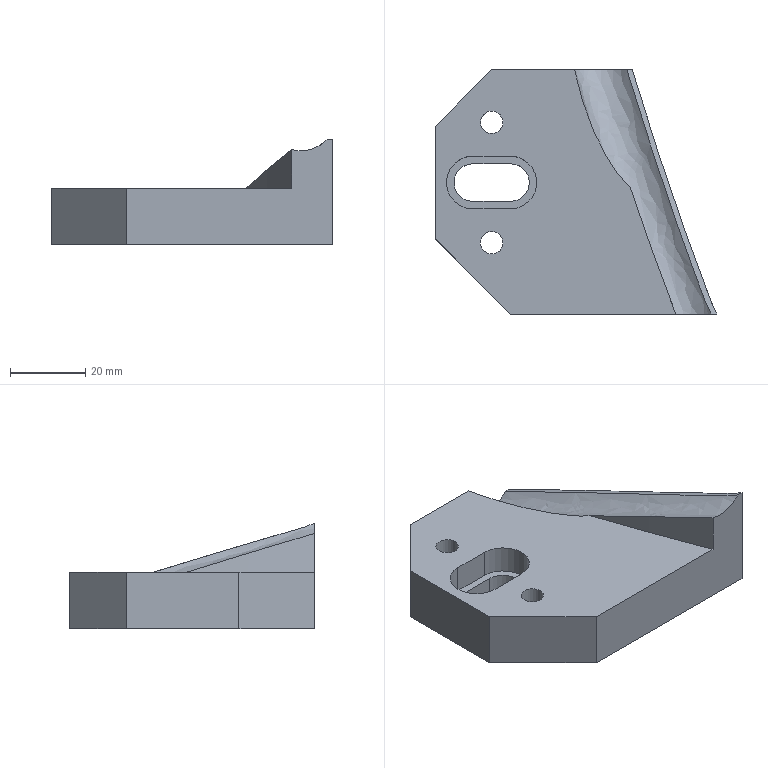Part | NX | features solid 2 | 1 solid | 22 faces | box 74.881 x 65 x 28.021 mm | volume 52689 mm3 | plane 12 | cylinder 6 | spline 4 | commonest cylinder face diameters 6 x2 10 x2 14 x2
STEP:
#1=CARTESIAN_POINT('',(-605.,-23.,-39.));
#2=VERTEX_POINT('',#1);
#3=CARTESIAN_POINT('',(-605.,-37.,-39.));
#4=VERTEX_POINT('',#3);
#5=CARTESIAN_POINT('',(-605.,-30.,-39.));
#6=DIRECTION('',(0.,0.,1.));
#7=DIRECTION('',(1.,0.,0.));
#8=AXIS2_PLACEMENT_3D('',#5,#6,#7);
#9=CIRCLE('',#8,7.);
#10=EDGE_CURVE('',#2,#4,#9,.T.);
#11=ORIENTED_EDGE('',*,*,#10,.F.);
#12=CARTESIAN_POINT('',(-595.,-23.,-39.));
#13=VERTEX_POINT('',#12);
#14=CARTESIAN_POINT('',(-558.,-23.,-39.));
#15=DIRECTION('',(1.,0.,0.));
#16=VECTOR('',#15,1000.);
#17=LINE('',#14,#16);
#18=EDGE_CURVE('',#2,#13,#17,.T.);
#19=ORIENTED_EDGE('',*,*,#18,.T.);
#20=CARTESIAN_POINT('',(-595.,-37.,-39.));
#21=VERTEX_POINT('',#20);
#22=CARTESIAN_POINT('',(-595.,-30.,-39.));
#23=DIRECTION('',(0.,0.,1.));
#24=DIRECTION('',(1.,0.,0.));
#25=AXIS2_PLACEMENT_3D('',#22,#23,#24);
#26=CIRCLE('',#25,7.);
#27=EDGE_CURVE('',#13,#21,#26,.F.);
#28=ORIENTED_EDGE('',*,*,#27,.T.);
#29=CARTESIAN_POINT('',(-558.,-37.,-39.));
#30=DIRECTION('',(1.,0.,0.));
#31=VECTOR('',#30,1000.);
#32=LINE('',#29,#31);
#33=EDGE_CURVE('',#4,#21,#32,.T.);
#34=ORIENTED_EDGE('',*,*,#33,.F.);
#35=EDGE_LOOP('',(#11,#19,#28,#34));
#36=FACE_BOUND('',#35,.T.);
#37=CARTESIAN_POINT('',(-597.,-46.,-39.));
#38=VERTEX_POINT('',#37);
#39=CARTESIAN_POINT('',(-600.,-46.,-39.));
#40=DIRECTION('',(0.,0.,1.));
#41=DIRECTION('',(1.,0.,0.));
#42=AXIS2_PLACEMENT_3D('',#39,#40,#41);
#43=CIRCLE('',#42,3.);
#44=EDGE_CURVE('',#38,#38,#43,.T.);
#45=ORIENTED_EDGE('',*,*,#44,.F.);
#46=EDGE_LOOP('',(#45));
#47=FACE_BOUND('',#46,.T.);
#48=CARTESIAN_POINT('',(-597.,-14.,-39.));
#49=VERTEX_POINT('',#48);
#50=CARTESIAN_POINT('',(-600.,-14.,-39.));
#51=DIRECTION('',(0.,0.,1.));
#52=DIRECTION('',(1.,0.,0.));
#53=AXIS2_PLACEMENT_3D('',#50,#51,#52);
#54=CIRCLE('',#53,3.);
#55=EDGE_CURVE('',#49,#49,#54,.T.);
#56=ORIENTED_EDGE('',*,*,#55,.F.);
#57=EDGE_LOOP('',(#56));
#58=FACE_BOUND('',#57,.T.);
#59=CARTESIAN_POINT('',(-577.951,0.,-39.));
#60=VERTEX_POINT('',#59);
#61=CARTESIAN_POINT('',(-600.,0.,-39.));
#62=VERTEX_POINT('',#61);
#63=CARTESIAN_POINT('',(-558.,0.,-39.));
#64=DIRECTION('',(-1.,0.,0.));
#65=VECTOR('',#64,1000.);
#66=LINE('',#63,#65);
#67=EDGE_CURVE('',#60,#62,#66,.T.);
#68=ORIENTED_EDGE('',*,*,#67,.T.);
#69=CARTESIAN_POINT('',(-615.,-15.,-39.));
#70=VERTEX_POINT('',#69);
#71=CARTESIAN_POINT('',(-606.5,-6.5,-39.));
#72=DIRECTION('',(-0.7071,-0.7071,0.));
#73=VECTOR('',#72,1000.);
#74=LINE('',#71,#73);
#75=EDGE_CURVE('',#62,#70,#74,.T.);
#76=ORIENTED_EDGE('',*,*,#75,.T.);
#77=CARTESIAN_POINT('',(-615.,-45.,-39.));
#78=VERTEX_POINT('',#77);
#79=CARTESIAN_POINT('',(-615.,-55.,-39.));
#80=DIRECTION('',(0.,-1.,0.));
#81=VECTOR('',#80,1000.);
#82=LINE('',#79,#81);
#83=EDGE_CURVE('',#70,#78,#82,.T.);
#84=ORIENTED_EDGE('',*,*,#83,.T.);
#85=CARTESIAN_POINT('',(-595.,-65.,-39.));
#86=VERTEX_POINT('',#85);
#87=CARTESIAN_POINT('',(-581.5,-78.5,-39.));
#88=DIRECTION('',(0.7071,-0.7071,0.));
#89=VECTOR('',#88,1000.);
#90=LINE('',#87,#89);
#91=EDGE_CURVE('',#78,#86,#90,.T.);
#92=ORIENTED_EDGE('',*,*,#91,.T.);
#93=CARTESIAN_POINT('',(-551.027,-65.,-39.));
#94=VERTEX_POINT('',#93);
#95=CARTESIAN_POINT('',(-606.945,-65.,-39.));
#96=DIRECTION('',(1.,0.,0.));
#97=VECTOR('',#96,1000.);
#98=LINE('',#95,#97);
#99=EDGE_CURVE('',#86,#94,#98,.T.);
#100=ORIENTED_EDGE('',*,*,#99,.T.);
#101=CARTESIAN_POINT('',(-563.215,-30.949,-39.));
#102=VERTEX_POINT('',#101);
#103=CARTESIAN_POINT('',(-563.215,-30.949,-39.));
#104=CARTESIAN_POINT('',(-561.296,-36.655,-39.));
#105=CARTESIAN_POINT('',(-557.402,-48.074,-39.));
#106=CARTESIAN_POINT('',(-553.142,-59.355,-39.));
#107=CARTESIAN_POINT('',(-551.027,-65.,-39.));
#108=B_SPLINE_CURVE_WITH_KNOTS('',3,(#103,#104,#105,#106,#107),.UNSPECIFIED.,.F.,.F.,(4,1,4),(0.1639,0.1818,0.1997),.UNSPECIFIED.);
#109=EDGE_CURVE('',#94,#102,#108,.F.);
#110=ORIENTED_EDGE('',*,*,#109,.T.);
#111=CARTESIAN_POINT('',(-577.951,0.,-39.));
#112=CARTESIAN_POINT('',(-577.382,-2.845,-39.));
#113=CARTESIAN_POINT('',(-575.919,-8.471,-39.));
#114=CARTESIAN_POINT('',(-572.885,-16.657,-39.));
#115=CARTESIAN_POINT('',(-569.649,-23.125,-39.));
#116=CARTESIAN_POINT('',(-566.404,-27.898,-39.));
#117=CARTESIAN_POINT('',(-564.4,-30.092,-39.));
#118=CARTESIAN_POINT('',(-563.215,-30.949,-39.));
#119=B_SPLINE_CURVE_WITH_KNOTS('',3,(#111,#112,#113,#114,#115,#116,#117,#118),.UNSPECIFIED.,.F.,.F.,(4,1,1,1,1,4),(0.01874,0.02746,0.03618,0.04491,0.04927,0.05363),.UNSPECIFIED.);
#120=EDGE_CURVE('',#102,#60,#119,.F.);
#121=ORIENTED_EDGE('',*,*,#120,.T.);
#122=EDGE_LOOP('',(#68,#76,#84,#92,#100,#110,#121));
#123=FACE_BOUND('',#122,.T.);
#124=CARTESIAN_POINT('',(-558.,-55.,-39.));
#125=DIRECTION('',(0.,0.,1.));
#126=DIRECTION('',(0.,-1.,0.));
#127=AXIS2_PLACEMENT_3D('',#124,#125,#126);
#128=PLANE('',#127);
#129=ADVANCED_FACE('',(#36,#47,#58,#123),#128,.T.);
#130=CARTESIAN_POINT('',(-595.,-25.,-46.5));
#131=VERTEX_POINT('',#130);
#132=CARTESIAN_POINT('',(-595.,-25.,-54.));
#133=VERTEX_POINT('',#132);
#134=CARTESIAN_POINT('',(-595.,-25.,-40.));
#135=DIRECTION('',(0.,0.,-1.));
#136=VECTOR('',#135,1000.);
#137=LINE('',#134,#136);
#138=EDGE_CURVE('',#131,#133,#137,.T.);
#139=ORIENTED_EDGE('',*,*,#138,.F.);
#140=CARTESIAN_POINT('',(-605.,-25.,-46.5));
#141=VERTEX_POINT('',#140);
#142=CARTESIAN_POINT('',(-595.,-25.,-46.5));
#143=DIRECTION('',(-1.,0.,0.));
#144=VECTOR('',#143,1000.);
#145=LINE('',#142,#144);
#146=EDGE_CURVE('',#131,#141,#145,.T.);
#147=ORIENTED_EDGE('',*,*,#146,.T.);
#148=CARTESIAN_POINT('',(-605.,-25.,-54.));
#149=VERTEX_POINT('',#148);
#150=CARTESIAN_POINT('',(-605.,-25.,-40.));
#151=DIRECTION('',(0.,0.,-1.));
#152=VECTOR('',#151,1000.);
#153=LINE('',#150,#152);
#154=EDGE_CURVE('',#141,#149,#153,.T.);
#155=ORIENTED_EDGE('',*,*,#154,.T.);
#156=CARTESIAN_POINT('',(-595.,-25.,-54.));
#157=DIRECTION('',(-1.,0.,0.));
#158=VECTOR('',#157,1000.);
#159=LINE('',#156,#158);
#160=EDGE_CURVE('',#133,#149,#159,.T.);
#161=ORIENTED_EDGE('',*,*,#160,.F.);
#162=EDGE_LOOP('',(#139,#147,#155,#161));
#163=FACE_BOUND('',#162,.T.);
#164=CARTESIAN_POINT('',(-595.,-25.,-40.));
#165=DIRECTION('',(0.,-1.,0.));
#166=DIRECTION('',(1.,0.,0.));
#167=AXIS2_PLACEMENT_3D('',#164,#165,#166);
#168=PLANE('',#167);
#169=ADVANCED_FACE('',(#163),#168,.T.);
#170=ORIENTED_EDGE('',*,*,#154,.F.);
#171=CARTESIAN_POINT('',(-605.,-35.,-46.5));
#172=VERTEX_POINT('',#171);
#173=CARTESIAN_POINT('',(-605.,-30.,-46.5));
#174=DIRECTION('',(0.,0.,1.));
#175=DIRECTION('',(0.,-1.,0.));
#176=AXIS2_PLACEMENT_3D('',#173,#174,#175);
#177=CIRCLE('',#176,5.);
#178=EDGE_CURVE('',#141,#172,#177,.T.);
#179=ORIENTED_EDGE('',*,*,#178,.T.);
#180=CARTESIAN_POINT('',(-605.,-35.,-54.));
#181=VERTEX_POINT('',#180);
#182=CARTESIAN_POINT('',(-605.,-35.,-40.));
#183=DIRECTION('',(0.,0.,-1.));
#184=VECTOR('',#183,1000.);
#185=LINE('',#182,#184);
#186=EDGE_CURVE('',#172,#181,#185,.T.);
#187=ORIENTED_EDGE('',*,*,#186,.T.);
#188=CARTESIAN_POINT('',(-605.,-30.,-54.));
#189=DIRECTION('',(0.,0.,1.));
#190=DIRECTION('',(1.,0.,0.));
#191=AXIS2_PLACEMENT_3D('',#188,#189,#190);
#192=CIRCLE('',#191,5.);
#193=EDGE_CURVE('',#149,#181,#192,.T.);
#194=ORIENTED_EDGE('',*,*,#193,.F.);
#195=EDGE_LOOP('',(#170,#179,#187,#194));
#196=FACE_BOUND('',#195,.T.);
#197=CARTESIAN_POINT('',(-605.,-30.,-40.));
#198=DIRECTION('',(0.,0.,-1.));
#199=DIRECTION('',(0.,1.,0.));
#200=AXIS2_PLACEMENT_3D('',#197,#198,#199);
#201=CYLINDRICAL_SURFACE('',#200,5.);
#202=ADVANCED_FACE('',(#196),#201,.F.);
#203=CARTESIAN_POINT('',(-595.,-35.,-46.5));
#204=VERTEX_POINT('',#203);
#205=CARTESIAN_POINT('',(-595.,-35.,-46.5));
#206=DIRECTION('',(-1.,0.,0.));
#207=VECTOR('',#206,1000.);
#208=LINE('',#205,#207);
#209=EDGE_CURVE('',#204,#172,#208,.T.);
#210=ORIENTED_EDGE('',*,*,#209,.F.);
#211=CARTESIAN_POINT('',(-595.,-35.,-54.));
#212=VERTEX_POINT('',#211);
#213=CARTESIAN_POINT('',(-595.,-35.,-40.));
#214=DIRECTION('',(0.,0.,-1.));
#215=VECTOR('',#214,1000.);
#216=LINE('',#213,#215);
#217=EDGE_CURVE('',#204,#212,#216,.T.);
#218=ORIENTED_EDGE('',*,*,#217,.T.);
#219=CARTESIAN_POINT('',(-595.,-35.,-54.));
#220=DIRECTION('',(-1.,0.,0.));
#221=VECTOR('',#220,1000.);
#222=LINE('',#219,#221);
#223=EDGE_CURVE('',#212,#181,#222,.T.);
#224=ORIENTED_EDGE('',*,*,#223,.T.);
#225=ORIENTED_EDGE('',*,*,#186,.F.);
#226=EDGE_LOOP('',(#210,#218,#224,#225));
#227=FACE_BOUND('',#226,.T.);
#228=CARTESIAN_POINT('',(-595.,-35.,-40.));
#229=DIRECTION('',(0.,-1.,0.));
#230=DIRECTION('',(1.,0.,0.));
#231=AXIS2_PLACEMENT_3D('',#228,#229,#230);
#232=PLANE('',#231);
#233=ADVANCED_FACE('',(#227),#232,.F.);
#234=ORIENTED_EDGE('',*,*,#217,.F.);
#235=CARTESIAN_POINT('',(-595.,-30.,-46.5));
#236=DIRECTION('',(0.,0.,1.));
#237=DIRECTION('',(0.,-1.,0.));
#238=AXIS2_PLACEMENT_3D('',#235,#236,#237);
#239=CIRCLE('',#238,5.);
#240=EDGE_CURVE('',#204,#131,#239,.T.);
#241=ORIENTED_EDGE('',*,*,#240,.T.);
#242=ORIENTED_EDGE('',*,*,#138,.T.);
#243=CARTESIAN_POINT('',(-595.,-30.,-54.));
#244=DIRECTION('',(0.,0.,1.));
#245=DIRECTION('',(1.,0.,0.));
#246=AXIS2_PLACEMENT_3D('',#243,#244,#245);
#247=CIRCLE('',#246,5.);
#248=EDGE_CURVE('',#212,#133,#247,.T.);
#249=ORIENTED_EDGE('',*,*,#248,.F.);
#250=EDGE_LOOP('',(#234,#241,#242,#249));
#251=FACE_BOUND('',#250,.T.);
#252=CARTESIAN_POINT('',(-595.,-30.,-40.));
#253=DIRECTION('',(0.,0.,-1.));
#254=DIRECTION('',(0.,1.,0.));
#255=AXIS2_PLACEMENT_3D('',#252,#253,#254);
#256=CYLINDRICAL_SURFACE('',#255,5.);
#257=ADVANCED_FACE('',(#251),#256,.F.);
#258=CARTESIAN_POINT('',(-540.119,-65.,-25.979));
#259=VERTEX_POINT('',#258);
#260=CARTESIAN_POINT('',(-562.627,0.,-46.096));
#261=VERTEX_POINT('',#260);
#262=CARTESIAN_POINT('',(-562.627,-0.000000076,-46.096));
#263=CARTESIAN_POINT('',(-562.476,-0.5056,-45.933));
#264=CARTESIAN_POINT('',(-562.046,-1.947,-45.468));
#265=CARTESIAN_POINT('',(-561.172,-4.822,-44.537));
#266=CARTESIAN_POINT('',(-560.26,-7.762,-43.584));
#267=CARTESIAN_POINT('',(-559.598,-9.867,-42.903));
#268=CARTESIAN_POINT('',(-559.013,-11.709,-42.307));
#269=CARTESIAN_POINT('',(-558.545,-13.172,-41.833));
#270=CARTESIAN_POINT('',(-558.133,-14.451,-41.42));
#271=CARTESIAN_POINT('',(-557.827,-15.395,-41.115));
#272=CARTESIAN_POINT('',(-557.656,-15.923,-40.945));
#273=CARTESIAN_POINT('',(-557.506,-16.384,-40.796));
#274=CARTESIAN_POINT('',(-557.429,-16.619,-40.721));
#275=CARTESIAN_POINT('',(-557.302,-17.01,-40.595));
#276=CARTESIAN_POINT('',(-557.092,-17.655,-40.387));
#277=CARTESIAN_POINT('',(-556.665,-18.957,-39.97));
#278=CARTESIAN_POINT('',(-556.069,-20.769,-39.392));
#279=CARTESIAN_POINT('',(-555.365,-22.893,-38.72));
#280=CARTESIAN_POINT('',(-554.447,-25.645,-37.858));
#281=CARTESIAN_POINT('',(-553.333,-28.966,-36.831));
#282=CARTESIAN_POINT('',(-552.09,-32.632,-35.721));
#283=CARTESIAN_POINT('',(-551.008,-35.788,-34.782));
#284=CARTESIAN_POINT('',(-550.047,-38.563,-33.963));
#285=CARTESIAN_POINT('',(-549.241,-40.87,-33.286));
#286=CARTESIAN_POINT('',(-548.548,-42.836,-32.711));
#287=CARTESIAN_POINT('',(-547.816,-44.894,-32.109));
#288=CARTESIAN_POINT('',(-547.212,-46.578,-31.616));
#289=CARTESIAN_POINT('',(-546.778,-47.777,-31.267));
#290=CARTESIAN_POINT('',(-546.539,-48.434,-31.075));
#291=CARTESIAN_POINT('',(-546.331,-49.003,-30.909));
#292=CARTESIAN_POINT('',(-546.23,-49.28,-30.828));
#293=CARTESIAN_POINT('',(-546.044,-49.788,-30.679));
#294=CARTESIAN_POINT('',(-545.708,-50.701,-30.409));
#295=CARTESIAN_POINT('',(-545.132,-52.252,-29.945));
#296=CARTESIAN_POINT('',(-544.449,-54.069,-29.399));
#297=CARTESIAN_POINT('',(-543.899,-55.518,-28.964));
#298=CARTESIAN_POINT('',(-543.582,-56.353,-28.715));
#299=CARTESIAN_POINT('',(-543.296,-57.104,-28.491));
#300=CARTESIAN_POINT('',(-543.152,-57.483,-28.379));
#301=CARTESIAN_POINT('',(-542.903,-58.142,-28.188));
#302=CARTESIAN_POINT('',(-542.47,-59.289,-27.862));
#303=CARTESIAN_POINT('',(-541.962,-60.695,-27.49));
#304=CARTESIAN_POINT('',(-541.343,-62.341,-27.031));
#305=CARTESIAN_POINT('',(-540.778,-63.709,-26.575));
#306=CARTESIAN_POINT('',(-540.368,-64.541,-26.222));
#307=CARTESIAN_POINT('',(-540.119,-65.,-25.979));
#308=B_SPLINE_CURVE_WITH_KNOTS('',3,(#262,#263,#264,#265,#266,#267,#268,#269,#270,#271,#272,#273,#274,#275,#276,#277,#278,#279,#280,#281,#282,#283,#284,#285,#286,#287,#288,#289,#290,#291,#292,#293,#294,#295,#296,#297,#298,#299,#300,#301,#302,#303,#304,#305,#306,#307),.UNSPECIFIED.,.F.,.F.,(4,1,1,1,1,1,1,1,1,1,1,1,1,1,1,1,1,1,1,1,1,1,1,1,1,1,1,1,1,1,1,1,1,1,1,1,1,1,1,1,1,1,1,4),(0.,0.0625,0.125,0.1562,0.1875,0.2031,0.2188,0.2344,0.2422,0.2461,0.25,0.2539,0.2578,0.2656,0.2812,0.3125,0.3438,0.375,0.4375,0.5,0.5625,0.5938,0.625,0.6562,0.6875,0.7188,0.7344,0.7422,0.75,0.7578,0.7656,0.7812,0.8125,0.8438,0.8594,0.8672,0.875,0.8828,0.8906,0.9062,0.9375,0.9531,0.9688,1.),.UNSPECIFIED.);
#309=EDGE_CURVE('',#259,#261,#308,.F.);
#310=ORIENTED_EDGE('',*,*,#309,.F.);
#311=CARTESIAN_POINT('',(-540.119,-65.,-54.));
#312=VERTEX_POINT('',#311);
#313=CARTESIAN_POINT('',(-540.119,-65.,-40.));
#314=DIRECTION('',(0.,0.,-1.));
#315=VECTOR('',#314,1000.);
#316=LINE('',#313,#315);
#317=EDGE_CURVE('',#259,#312,#316,.T.);
#318=ORIENTED_EDGE('',*,*,#317,.T.);
#319=CARTESIAN_POINT('',(-562.627,0.,-54.));
#320=VERTEX_POINT('',#319);
#321=CARTESIAN_POINT('',(-562.627,0.,-54.));
#322=CARTESIAN_POINT('',(-561.956,-2.253,-54.));
#323=CARTESIAN_POINT('',(-560.511,-6.995,-54.));
#324=CARTESIAN_POINT('',(-558.027,-14.816,-54.));
#325=CARTESIAN_POINT('',(-555.698,-21.916,-54.));
#326=CARTESIAN_POINT('',(-553.927,-27.206,-54.));
#327=CARTESIAN_POINT('',(-552.881,-30.299,-54.));
#328=CARTESIAN_POINT('',(-551.787,-33.518,-54.));
#329=CARTESIAN_POINT('',(-550.531,-37.176,-54.));
#330=CARTESIAN_POINT('',(-549.063,-41.385,-54.));
#331=CARTESIAN_POINT('',(-547.898,-44.672,-54.));
#332=CARTESIAN_POINT('',(-547.012,-47.134,-54.));
#333=CARTESIAN_POINT('',(-546.44,-48.708,-54.));
#334=CARTESIAN_POINT('',(-546.066,-49.727,-54.));
#335=CARTESIAN_POINT('',(-545.638,-50.886,-54.));
#336=CARTESIAN_POINT('',(-545.051,-52.461,-54.));
#337=CARTESIAN_POINT('',(-544.379,-54.245,-54.));
#338=CARTESIAN_POINT('',(-543.872,-55.586,-54.));
#339=CARTESIAN_POINT('',(-543.603,-56.297,-54.));
#340=CARTESIAN_POINT('',(-543.454,-56.688,-54.));
#341=CARTESIAN_POINT('',(-543.318,-57.047,-54.));
#342=CARTESIAN_POINT('',(-543.27,-57.172,-54.));
#343=CARTESIAN_POINT('',(-543.169,-57.438,-54.));
#344=CARTESIAN_POINT('',(-542.996,-57.898,-54.));
#345=CARTESIAN_POINT('',(-542.703,-58.682,-54.));
#346=CARTESIAN_POINT('',(-542.304,-59.753,-54.));
#347=CARTESIAN_POINT('',(-541.665,-61.501,-54.));
#348=CARTESIAN_POINT('',(-540.929,-63.376,-54.));
#349=CARTESIAN_POINT('',(-540.381,-64.517,-54.));
#350=CARTESIAN_POINT('',(-540.119,-65.,-54.));
#351=B_SPLINE_CURVE_WITH_KNOTS('',3,(#321,#322,#323,#324,#325,#326,#327,#328,#329,#330,#331,#332,#333,#334,#335,#336,#337,#338,#339,#340,#341,#342,#343,#344,#345,#346,#347,#348,#349,#350),.UNSPECIFIED.,.F.,.F.,(4,1,1,1,1,1,1,1,1,1,1,1,1,1,1,1,1,1,1,1,1,1,1,1,1,1,1,4),(0.,0.125,0.25,0.375,0.4375,0.4688,0.5,0.5625,0.625,0.6875,0.7188,0.75,0.7656,0.7812,0.8125,0.8438,0.8594,0.8672,0.8711,0.875,0.8789,0.8828,0.8906,0.9062,0.9219,0.9375,0.9688,1.),.UNSPECIFIED.);
#352=EDGE_CURVE('',#320,#312,#351,.T.);
#353=ORIENTED_EDGE('',*,*,#352,.F.);
#354=CARTESIAN_POINT('',(-562.627,0.,-40.));
#355=DIRECTION('',(0.,0.,-1.));
#356=VECTOR('',#355,1000.);
#357=LINE('',#354,#356);
#358=EDGE_CURVE('',#261,#320,#357,.T.);
#359=ORIENTED_EDGE('',*,*,#358,.F.);
#360=EDGE_LOOP('',(#310,#318,#353,#359));
#361=FACE_BOUND('',#360,.T.);
#362=CARTESIAN_POINT('',(-562.627,0.,-45.852));
#363=CARTESIAN_POINT('',(-562.627,0.,-74.588));
#364=CARTESIAN_POINT('',(-560.996,-5.48,-44.093));
#365=CARTESIAN_POINT('',(-560.996,-5.48,-72.83));
#366=CARTESIAN_POINT('',(-557.555,-16.391,-40.592));
#367=CARTESIAN_POINT('',(-557.555,-16.391,-69.329));
#368=CARTESIAN_POINT('',(-553.012,-29.979,-36.299));
#369=CARTESIAN_POINT('',(-553.012,-29.979,-65.036));
#370=CARTESIAN_POINT('',(-549.272,-40.823,-32.902));
#371=CARTESIAN_POINT('',(-549.272,-40.823,-61.639));
#372=CARTESIAN_POINT('',(-546.863,-47.577,-30.783));
#373=CARTESIAN_POINT('',(-546.863,-47.577,-59.519));
#374=CARTESIAN_POINT('',(-544.875,-52.963,-29.101));
#375=CARTESIAN_POINT('',(-544.875,-52.963,-57.838));
#376=CARTESIAN_POINT('',(-543.328,-56.989,-27.867));
#377=CARTESIAN_POINT('',(-543.328,-56.989,-56.603));
#378=CARTESIAN_POINT('',(-541.841,-61.043,-26.646));
#379=CARTESIAN_POINT('',(-541.841,-61.043,-55.382));
#380=CARTESIAN_POINT('',(-540.806,-63.733,-25.833));
#381=CARTESIAN_POINT('',(-540.806,-63.733,-54.57));
#382=CARTESIAN_POINT('',(-540.119,-65.,-25.434));
#383=CARTESIAN_POINT('',(-540.119,-65.,-54.17));
#384=B_SPLINE_SURFACE_WITH_KNOTS('',3,1,((#362,#363),(#364,#365),(#366,#367),(#368,#369),(#370,#371),(#372,#373),(#374,#375),(#376,#377),(#378,#379),(#380,#381),(#382,#383)),.SURF_OF_LINEAR_EXTRUSION.,.F.,.F.,.F.,(4,1,1,1,1,1,1,1,4),(2,2),(0.626,0.6508,0.6755,0.6879,0.7003,0.7065,0.7127,0.7189,0.7251),(0.,1.),.UNSPECIFIED.);
#385=ADVANCED_FACE('',(#361),#384,.T.);
#386=ORIENTED_EDGE('',*,*,#317,.F.);
#387=CARTESIAN_POINT('',(-541.633,-65.,-25.979));
#388=VERTEX_POINT('',#387);
#389=CARTESIAN_POINT('',(-540.416,-65.,-25.979));
#390=DIRECTION('',(-1.,0.,0.));
#391=VECTOR('',#390,1000.);
#392=LINE('',#389,#391);
#393=EDGE_CURVE('',#259,#388,#392,.T.);
#394=ORIENTED_EDGE('',*,*,#393,.T.);
#395=CARTESIAN_POINT('',(-551.027,-65.,-28.683));
#396=VERTEX_POINT('',#395);
#397=CARTESIAN_POINT('',(-551.027,-65.,-28.683));
#398=CARTESIAN_POINT('',(-547.719,-65.,-29.71));
#399=CARTESIAN_POINT('',(-543.963,-65.,-28.474));
#400=CARTESIAN_POINT('',(-541.633,-65.,-25.979));
#401=B_SPLINE_CURVE_WITH_KNOTS('',3,(#397,#398,#399,#400),.UNSPECIFIED.,.F.,.F.,(4,4),(0.,0.01028),.UNSPECIFIED.);
#402=EDGE_CURVE('',#396,#388,#401,.T.);
#403=ORIENTED_EDGE('',*,*,#402,.F.);
#404=CARTESIAN_POINT('',(-551.027,-65.,-32.5));
#405=DIRECTION('',(0.,0.,-1.));
#406=VECTOR('',#405,1000.);
#407=LINE('',#404,#406);
#408=EDGE_CURVE('',#396,#94,#407,.T.);
#409=ORIENTED_EDGE('',*,*,#408,.T.);
#410=ORIENTED_EDGE('',*,*,#99,.F.);
#411=CARTESIAN_POINT('',(-595.,-65.,-54.));
#412=VERTEX_POINT('',#411);
#413=CARTESIAN_POINT('',(-595.,-65.,-40.));
#414=DIRECTION('',(0.,0.,-1.));
#415=VECTOR('',#414,1000.);
#416=LINE('',#413,#415);
#417=EDGE_CURVE('',#86,#412,#416,.T.);
#418=ORIENTED_EDGE('',*,*,#417,.T.);
#419=CARTESIAN_POINT('',(-606.945,-65.,-54.));
#420=DIRECTION('',(1.,0.,0.));
#421=VECTOR('',#420,1000.);
#422=LINE('',#419,#421);
#423=EDGE_CURVE('',#412,#312,#422,.T.);
#424=ORIENTED_EDGE('',*,*,#423,.T.);
#425=EDGE_LOOP('',(#386,#394,#403,#409,#410,#418,#424));
#426=FACE_BOUND('',#425,.T.);
#427=CARTESIAN_POINT('',(-606.945,-65.,-40.));
#428=DIRECTION('',(0.,1.,0.));
#429=DIRECTION('',(0.,0.,1.));
#430=AXIS2_PLACEMENT_3D('',#427,#428,#429);
#431=PLANE('',#430);
#432=ADVANCED_FACE('',(#426),#431,.F.);
#433=ORIENTED_EDGE('',*,*,#44,.T.);
#434=EDGE_LOOP('',(#433));
#435=FACE_BOUND('',#434,.T.);
#436=CARTESIAN_POINT('',(-597.,-46.,-54.));
#437=VERTEX_POINT('',#436);
#438=CARTESIAN_POINT('',(-600.,-46.,-54.));
#439=DIRECTION('',(0.,0.,1.));
#440=DIRECTION('',(1.,0.,0.));
#441=AXIS2_PLACEMENT_3D('',#438,#439,#440);
#442=CIRCLE('',#441,3.);
#443=EDGE_CURVE('',#437,#437,#442,.T.);
#444=ORIENTED_EDGE('',*,*,#443,.F.);
#445=EDGE_LOOP('',(#444));
#446=FACE_BOUND('',#445,.T.);
#447=CARTESIAN_POINT('',(-600.,-46.,-40.));
#448=DIRECTION('',(0.,0.,-1.));
#449=DIRECTION('',(0.,1.,0.));
#450=AXIS2_PLACEMENT_3D('',#447,#448,#449);
#451=CYLINDRICAL_SURFACE('',#450,3.);
#452=ADVANCED_FACE('',(#435,#446),#451,.F.);
#453=CARTESIAN_POINT('',(-564.061,0.,-46.096));
#454=VERTEX_POINT('',#453);
#455=CARTESIAN_POINT('',(-564.061,0.,-46.096));
#456=CARTESIAN_POINT('',(-565.296,0.,-47.443));
#457=CARTESIAN_POINT('',(-568.554,0.,-49.428));
#458=CARTESIAN_POINT('',(-574.364,0.,-48.967));
#459=CARTESIAN_POINT('',(-578.369,0.,-44.645));
#460=CARTESIAN_POINT('',(-578.456,0.,-40.758));
#461=CARTESIAN_POINT('',(-577.951,0.,-39.));
#462=B_SPLINE_CURVE_WITH_KNOTS('',3,(#455,#456,#457,#458,#459,#460,#461),.UNSPECIFIED.,.F.,.F.,(4,1,1,1,4),(0.002501,0.007958,0.01342,0.01887,0.02433),.UNSPECIFIED.);
#463=EDGE_CURVE('',#454,#60,#462,.T.);
#464=ORIENTED_EDGE('',*,*,#463,.F.);
#465=CARTESIAN_POINT('',(-564.061,0.,-46.096));
#466=DIRECTION('',(-1.,0.,0.));
#467=VECTOR('',#466,1000.);
#468=LINE('',#465,#467);
#469=EDGE_CURVE('',#454,#261,#468,.F.);
#470=ORIENTED_EDGE('',*,*,#469,.T.);
#471=ORIENTED_EDGE('',*,*,#358,.T.);
#472=CARTESIAN_POINT('',(-600.,0.,-54.));
#473=VERTEX_POINT('',#472);
#474=CARTESIAN_POINT('',(-558.,0.,-54.));
#475=DIRECTION('',(-1.,0.,0.));
#476=VECTOR('',#475,1000.);
#477=LINE('',#474,#476);
#478=EDGE_CURVE('',#320,#473,#477,.T.);
#479=ORIENTED_EDGE('',*,*,#478,.T.);
#480=CARTESIAN_POINT('',(-600.,0.,-43.));
#481=DIRECTION('',(0.,0.,1.));
#482=VECTOR('',#481,1000.);
#483=LINE('',#480,#482);
#484=EDGE_CURVE('',#473,#62,#483,.T.);
#485=ORIENTED_EDGE('',*,*,#484,.T.);
#486=ORIENTED_EDGE('',*,*,#67,.F.);
#487=EDGE_LOOP('',(#464,#470,#471,#479,#485,#486));
#488=FACE_BOUND('',#487,.T.);
#489=CARTESIAN_POINT('',(-558.,0.,-40.));
#490=DIRECTION('',(0.,-1.,0.));
#491=DIRECTION('',(1.,0.,0.));
#492=AXIS2_PLACEMENT_3D('',#489,#490,#491);
#493=PLANE('',#492);
#494=ADVANCED_FACE('',(#488),#493,.F.);
#495=ORIENTED_EDGE('',*,*,#55,.T.);
#496=EDGE_LOOP('',(#495));
#497=FACE_BOUND('',#496,.T.);
#498=CARTESIAN_POINT('',(-597.,-14.,-54.));
#499=VERTEX_POINT('',#498);
#500=CARTESIAN_POINT('',(-600.,-14.,-54.));
#501=DIRECTION('',(0.,0.,1.));
#502=DIRECTION('',(1.,0.,0.));
#503=AXIS2_PLACEMENT_3D('',#500,#501,#502);
#504=CIRCLE('',#503,3.);
#505=EDGE_CURVE('',#499,#499,#504,.T.);
#506=ORIENTED_EDGE('',*,*,#505,.F.);
#507=EDGE_LOOP('',(#506));
#508=FACE_BOUND('',#507,.T.);
#509=CARTESIAN_POINT('',(-600.,-14.,-40.));
#510=DIRECTION('',(0.,0.,-1.));
#511=DIRECTION('',(0.,1.,0.));
#512=AXIS2_PLACEMENT_3D('',#509,#510,#511);
#513=CYLINDRICAL_SURFACE('',#512,3.);
#514=ADVANCED_FACE('',(#497,#508),#513,.F.);
#515=CARTESIAN_POINT('',(-615.,-15.,-54.));
#516=VERTEX_POINT('',#515);
#517=CARTESIAN_POINT('',(-615.,-45.,-54.));
#518=VERTEX_POINT('',#517);
#519=CARTESIAN_POINT('',(-615.,-55.,-54.));
#520=DIRECTION('',(0.,-1.,0.));
#521=VECTOR('',#520,1000.);
#522=LINE('',#519,#521);
#523=EDGE_CURVE('',#516,#518,#522,.T.);
#524=ORIENTED_EDGE('',*,*,#523,.F.);
#525=CARTESIAN_POINT('',(-615.,-15.,-54.));
#526=DIRECTION('',(0.7071,0.7071,0.));
#527=VECTOR('',#526,1000.);
#528=LINE('',#525,#527);
#529=EDGE_CURVE('',#516,#473,#528,.T.);
#530=ORIENTED_EDGE('',*,*,#529,.T.);
#531=ORIENTED_EDGE('',*,*,#478,.F.);
#532=ORIENTED_EDGE('',*,*,#352,.T.);
#533=ORIENTED_EDGE('',*,*,#423,.F.);
#534=CARTESIAN_POINT('',(-605.,-55.,-54.));
#535=DIRECTION('',(-0.7071,0.7071,0.));
#536=VECTOR('',#535,1000.);
#537=LINE('',#534,#536);
#538=EDGE_CURVE('',#412,#518,#537,.T.);
#539=ORIENTED_EDGE('',*,*,#538,.T.);
#540=EDGE_LOOP('',(#524,#530,#531,#532,#533,#539));
#541=FACE_BOUND('',#540,.T.);
#542=ORIENTED_EDGE('',*,*,#505,.T.);
#543=EDGE_LOOP('',(#542));
#544=FACE_BOUND('',#543,.T.);
#545=ORIENTED_EDGE('',*,*,#443,.T.);
#546=EDGE_LOOP('',(#545));
#547=FACE_BOUND('',#546,.T.);
#548=ORIENTED_EDGE('',*,*,#160,.T.);
#549=ORIENTED_EDGE('',*,*,#193,.T.);
#550=ORIENTED_EDGE('',*,*,#223,.F.);
#551=ORIENTED_EDGE('',*,*,#248,.T.);
#552=EDGE_LOOP('',(#548,#549,#550,#551));
#553=FACE_BOUND('',#552,.T.);
#554=CARTESIAN_POINT('',(-558.,-55.,-54.));
#555=DIRECTION('',(0.,0.,1.));
#556=DIRECTION('',(0.,-1.,0.));
#557=AXIS2_PLACEMENT_3D('',#554,#555,#556);
#558=PLANE('',#557);
#559=ADVANCED_FACE('',(#541,#544,#547,#553),#558,.F.);
#560=CARTESIAN_POINT('',(-605.,-23.,-46.5));
#561=VERTEX_POINT('',#560);
#562=CARTESIAN_POINT('',(-605.,-23.,-38.));
#563=DIRECTION('',(0.,0.,-1.));
#564=VECTOR('',#563,1000.);
#565=LINE('',#562,#564);
#566=EDGE_CURVE('',#2,#561,#565,.T.);
#567=ORIENTED_EDGE('',*,*,#566,.T.);
#568=CARTESIAN_POINT('',(-595.,-23.,-46.5));
#569=VERTEX_POINT('',#568);
#570=CARTESIAN_POINT('',(-595.,-23.,-46.5));
#571=DIRECTION('',(-1.,0.,0.));
#572=VECTOR('',#571,1000.);
#573=LINE('',#570,#572);
#574=EDGE_CURVE('',#569,#561,#573,.T.);
#575=ORIENTED_EDGE('',*,*,#574,.F.);
#576=CARTESIAN_POINT('',(-595.,-23.,-38.));
#577=DIRECTION('',(0.,0.,-1.));
#578=VECTOR('',#577,1000.);
#579=LINE('',#576,#578);
#580=EDGE_CURVE('',#13,#569,#579,.T.);
#581=ORIENTED_EDGE('',*,*,#580,.F.);
#582=ORIENTED_EDGE('',*,*,#18,.F.);
#583=EDGE_LOOP('',(#567,#575,#581,#582));
#584=FACE_BOUND('',#583,.T.);
#585=CARTESIAN_POINT('',(-595.,-23.,-38.));
#586=DIRECTION('',(0.,-1.,0.));
#587=DIRECTION('',(0.,0.,-1.));
#588=AXIS2_PLACEMENT_3D('',#585,#586,#587);
#589=PLANE('',#588);
#590=ADVANCED_FACE('',(#584),#589,.T.);
#591=ORIENTED_EDGE('',*,*,#10,.T.);
#592=CARTESIAN_POINT('',(-605.,-37.,-46.5));
#593=VERTEX_POINT('',#592);
#594=CARTESIAN_POINT('',(-605.,-37.,-38.));
#595=DIRECTION('',(0.,0.,-1.));
#596=VECTOR('',#595,1000.);
#597=LINE('',#594,#596);
#598=EDGE_CURVE('',#4,#593,#597,.T.);
#599=ORIENTED_EDGE('',*,*,#598,.T.);
#600=CARTESIAN_POINT('',(-605.,-30.,-46.5));
#601=DIRECTION('',(0.,0.,-1.));
#602=DIRECTION('',(0.,1.,0.));
#603=AXIS2_PLACEMENT_3D('',#600,#601,#602);
#604=CIRCLE('',#603,7.);
#605=EDGE_CURVE('',#593,#561,#604,.T.);
#606=ORIENTED_EDGE('',*,*,#605,.T.);
#607=ORIENTED_EDGE('',*,*,#566,.F.);
#608=EDGE_LOOP('',(#591,#599,#606,#607));
#609=FACE_BOUND('',#608,.T.);
#610=CARTESIAN_POINT('',(-605.,-30.,-38.));
#611=DIRECTION('',(0.,0.,-1.));
#612=DIRECTION('',(0.,1.,0.));
#613=AXIS2_PLACEMENT_3D('',#610,#611,#612);
#614=CYLINDRICAL_SURFACE('',#613,7.);
#615=ADVANCED_FACE('',(#609),#614,.F.);
#616=ORIENTED_EDGE('',*,*,#33,.T.);
#617=CARTESIAN_POINT('',(-595.,-37.,-46.5));
#618=VERTEX_POINT('',#617);
#619=CARTESIAN_POINT('',(-595.,-37.,-38.));
#620=DIRECTION('',(0.,0.,-1.));
#621=VECTOR('',#620,1000.);
#622=LINE('',#619,#621);
#623=EDGE_CURVE('',#21,#618,#622,.T.);
#624=ORIENTED_EDGE('',*,*,#623,.T.);
#625=CARTESIAN_POINT('',(-595.,-37.,-46.5));
#626=DIRECTION('',(-1.,0.,0.));
#627=VECTOR('',#626,1000.);
#628=LINE('',#625,#627);
#629=EDGE_CURVE('',#618,#593,#628,.T.);
#630=ORIENTED_EDGE('',*,*,#629,.T.);
#631=ORIENTED_EDGE('',*,*,#598,.F.);
#632=EDGE_LOOP('',(#616,#624,#630,#631));
#633=FACE_BOUND('',#632,.T.);
#634=CARTESIAN_POINT('',(-595.,-37.,-38.));
#635=DIRECTION('',(0.,-1.,0.));
#636=DIRECTION('',(1.,0.,0.));
#637=AXIS2_PLACEMENT_3D('',#634,#635,#636);
#638=PLANE('',#637);
#639=ADVANCED_FACE('',(#633),#638,.F.);
#640=ORIENTED_EDGE('',*,*,#580,.T.);
#641=CARTESIAN_POINT('',(-595.,-30.,-46.5));
#642=DIRECTION('',(0.,0.,1.));
#643=DIRECTION('',(0.,-1.,0.));
#644=AXIS2_PLACEMENT_3D('',#641,#642,#643);
#645=CIRCLE('',#644,7.);
#646=EDGE_CURVE('',#618,#569,#645,.T.);
#647=ORIENTED_EDGE('',*,*,#646,.F.);
#648=ORIENTED_EDGE('',*,*,#623,.F.);
#649=ORIENTED_EDGE('',*,*,#27,.F.);
#650=EDGE_LOOP('',(#640,#647,#648,#649));
#651=FACE_BOUND('',#650,.T.);
#652=CARTESIAN_POINT('',(-595.,-30.,-38.));
#653=DIRECTION('',(0.,0.,-1.));
#654=DIRECTION('',(0.,1.,0.));
#655=AXIS2_PLACEMENT_3D('',#652,#653,#654);
#656=CYLINDRICAL_SURFACE('',#655,7.);
#657=ADVANCED_FACE('',(#651),#656,.F.);
#658=ORIENTED_EDGE('',*,*,#240,.F.);
#659=ORIENTED_EDGE('',*,*,#209,.T.);
#660=ORIENTED_EDGE('',*,*,#178,.F.);
#661=ORIENTED_EDGE('',*,*,#146,.F.);
#662=EDGE_LOOP('',(#658,#659,#660,#661));
#663=FACE_BOUND('',#662,.T.);
#664=ORIENTED_EDGE('',*,*,#574,.T.);
#665=ORIENTED_EDGE('',*,*,#605,.F.);
#666=ORIENTED_EDGE('',*,*,#629,.F.);
#667=ORIENTED_EDGE('',*,*,#646,.T.);
#668=EDGE_LOOP('',(#664,#665,#666,#667));
#669=FACE_BOUND('',#668,.T.);
#670=CARTESIAN_POINT('',(-605.,-30.,-46.5));
#671=DIRECTION('',(0.,0.,1.));
#672=DIRECTION('',(0.,-1.,0.));
#673=AXIS2_PLACEMENT_3D('',#670,#671,#672);
#674=PLANE('',#673);
#675=ADVANCED_FACE('',(#663,#669),#674,.T.);
#676=CARTESIAN_POINT('',(-563.215,-30.949,-39.));
#677=CARTESIAN_POINT('',(-561.298,-36.649,-37.234));
#678=CARTESIAN_POINT('',(-557.414,-48.04,-33.723));
#679=CARTESIAN_POINT('',(-553.147,-59.341,-30.353));
#680=CARTESIAN_POINT('',(-551.027,-65.,-28.683));
#681=B_SPLINE_CURVE_WITH_KNOTS('',3,(#676,#677,#678,#679,#680),.UNSPECIFIED.,.F.,.F.,(4,1,4),(0.0339,0.05271,0.07152),.UNSPECIFIED.);
#682=EDGE_CURVE('',#102,#396,#681,.T.);
#683=ORIENTED_EDGE('',*,*,#682,.F.);
#684=ORIENTED_EDGE('',*,*,#109,.F.);
#685=ORIENTED_EDGE('',*,*,#408,.F.);
#686=EDGE_LOOP('',(#683,#684,#685));
#687=FACE_BOUND('',#686,.T.);
#688=CARTESIAN_POINT('',(-563.283,-30.744,-39.001));
#689=CARTESIAN_POINT('',(-563.283,-30.744,-49.62));
#690=CARTESIAN_POINT('',(-562.321,-33.607,-38.105));
#691=CARTESIAN_POINT('',(-562.321,-33.607,-48.724));
#692=CARTESIAN_POINT('',(-560.374,-39.338,-36.322));
#693=CARTESIAN_POINT('',(-560.374,-39.338,-46.941));
#694=CARTESIAN_POINT('',(-557.871,-46.496,-34.102));
#695=CARTESIAN_POINT('',(-557.871,-46.496,-44.721));
#696=CARTESIAN_POINT('',(-555.802,-52.24,-32.332));
#697=CARTESIAN_POINT('',(-555.802,-52.24,-42.951));
#698=CARTESIAN_POINT('',(-554.208,-56.549,-31.012));
#699=CARTESIAN_POINT('',(-554.208,-56.549,-41.631));
#700=CARTESIAN_POINT('',(-552.837,-60.145,-29.935));
#701=CARTESIAN_POINT('',(-552.837,-60.145,-40.554));
#702=CARTESIAN_POINT('',(-551.812,-62.848,-29.086));
#703=CARTESIAN_POINT('',(-551.812,-62.848,-39.705));
#704=CARTESIAN_POINT('',(-551.328,-64.196,-28.658));
#705=CARTESIAN_POINT('',(-551.328,-64.196,-39.277));
#706=CARTESIAN_POINT('',(-551.027,-65.,-28.444));
#707=CARTESIAN_POINT('',(-551.027,-65.,-39.063));
#708=B_SPLINE_SURFACE_WITH_KNOTS('',3,1,((#688,#689),(#690,#691),(#692,#693),(#694,#695),(#696,#697),(#698,#699),(#700,#701),(#702,#703),(#704,#705),(#706,#707)),.SURF_OF_LINEAR_EXTRUSION.,.F.,.F.,.F.,(4,1,1,1,1,1,1,4),(2,2),(0.6677,0.6807,0.6936,0.7001,0.7066,0.7131,0.7163,0.7196),(0.,1.),.UNSPECIFIED.);
#709=ADVANCED_FACE('',(#687),#708,.F.);
#710=CARTESIAN_POINT('',(-564.061,0.,-46.096));
#711=CARTESIAN_POINT('',(-562.435,-5.476,-44.335));
#712=CARTESIAN_POINT('',(-559.851,-13.635,-41.671));
#713=CARTESIAN_POINT('',(-556.246,-24.489,-38.196));
#714=CARTESIAN_POINT('',(-553.519,-32.658,-35.702));
#715=CARTESIAN_POINT('',(-550.744,-40.837,-33.291));
#716=CARTESIAN_POINT('',(-548.362,-47.637,-31.314));
#717=CARTESIAN_POINT('',(-546.386,-53.041,-29.72));
#718=CARTESIAN_POINT('',(-544.833,-57.045,-28.482));
#719=CARTESIAN_POINT('',(-543.378,-61.146,-27.377));
#720=CARTESIAN_POINT('',(-542.338,-63.832,-26.596));
#721=CARTESIAN_POINT('',(-541.633,-65.,-25.979));
#722=B_SPLINE_CURVE_WITH_KNOTS('',3,(#710,#711,#712,#713,#714,#715,#716,#717,#718,#719,#720,#721),.UNSPECIFIED.,.F.,.F.,(4,1,1,1,1,1,1,1,1,4),(0.08893,0.1068,0.1158,0.1248,0.1337,0.1427,0.1472,0.1517,0.1561,0.1606),.UNSPECIFIED.);
#723=EDGE_CURVE('',#454,#388,#722,.T.);
#724=ORIENTED_EDGE('',*,*,#723,.F.);
#725=ORIENTED_EDGE('',*,*,#463,.T.);
#726=ORIENTED_EDGE('',*,*,#120,.F.);
#727=ORIENTED_EDGE('',*,*,#682,.T.);
#728=ORIENTED_EDGE('',*,*,#402,.T.);
#729=EDGE_LOOP('',(#724,#725,#726,#727,#728));
#730=FACE_BOUND('',#729,.T.);
#731=CARTESIAN_POINT('',(-564.918,3.684,-47.028));
#732=CARTESIAN_POINT('',(-565.202,3.506,-47.33));
#733=CARTESIAN_POINT('',(-565.77,3.151,-47.934));
#734=CARTESIAN_POINT('',(-567.165,2.455,-48.859));
#735=CARTESIAN_POINT('',(-569.187,1.654,-49.547));
#736=CARTESIAN_POINT('',(-571.829,0.9125,-49.493));
#737=CARTESIAN_POINT('',(-574.374,0.4738,-48.574));
#738=CARTESIAN_POINT('',(-576.539,0.3879,-46.893));
#739=CARTESIAN_POINT('',(-578.08,0.6638,-44.64));
#740=CARTESIAN_POINT('',(-578.688,1.171,-42.5));
#741=CARTESIAN_POINT('',(-578.754,1.705,-40.769));
#742=CARTESIAN_POINT('',(-578.603,2.014,-39.935));
#743=CARTESIAN_POINT('',(-578.527,2.169,-39.518));
#744=CARTESIAN_POINT('',(-564.067,0.8007,-46.1));
#745=CARTESIAN_POINT('',(-564.35,0.6219,-46.402));
#746=CARTESIAN_POINT('',(-564.915,0.2642,-47.004));
#747=CARTESIAN_POINT('',(-566.303,-0.4369,-47.927));
#748=CARTESIAN_POINT('',(-568.316,-1.246,-48.615));
#749=CARTESIAN_POINT('',(-570.947,-2.001,-48.565));
#750=CARTESIAN_POINT('',(-573.486,-2.454,-47.654));
#751=CARTESIAN_POINT('',(-575.649,-2.555,-45.983));
#752=CARTESIAN_POINT('',(-577.196,-2.293,-43.74));
#753=CARTESIAN_POINT('',(-577.815,-1.794,-41.607));
#754=CARTESIAN_POINT('',(-577.892,-1.266,-39.879));
#755=CARTESIAN_POINT('',(-577.747,-0.9576,-39.046));
#756=CARTESIAN_POINT('',(-577.675,-0.8036,-38.629));
#757=CARTESIAN_POINT('',(-562.366,-4.967,-44.244));
#758=CARTESIAN_POINT('',(-562.646,-5.147,-44.544));
#759=CARTESIAN_POINT('',(-563.205,-5.509,-45.144));
#760=CARTESIAN_POINT('',(-564.579,-6.22,-46.064));
#761=CARTESIAN_POINT('',(-566.573,-7.046,-46.752));
#762=CARTESIAN_POINT('',(-569.184,-7.827,-46.71));
#763=CARTESIAN_POINT('',(-571.709,-8.31,-45.815));
#764=CARTESIAN_POINT('',(-573.87,-8.441,-44.163));
#765=CARTESIAN_POINT('',(-575.429,-8.206,-41.94));
#766=CARTESIAN_POINT('',(-576.068,-7.725,-39.821));
#767=CARTESIAN_POINT('',(-576.168,-7.206,-38.099));
#768=CARTESIAN_POINT('',(-576.037,-6.901,-37.267));
#769=CARTESIAN_POINT('',(-575.971,-6.748,-36.851));
#770=CARTESIAN_POINT('',(-558.756,-16.492,-40.558));
#771=CARTESIAN_POINT('',(-559.03,-16.673,-40.855));
#772=CARTESIAN_POINT('',(-559.579,-17.036,-41.45));
#773=CARTESIAN_POINT('',(-560.927,-17.755,-42.367));
#774=CARTESIAN_POINT('',(-562.885,-18.599,-43.061));
#775=CARTESIAN_POINT('',(-565.456,-19.416,-43.043));
#776=CARTESIAN_POINT('',(-567.955,-19.946,-42.186));
#777=CARTESIAN_POINT('',(-570.112,-20.131,-40.581));
#778=CARTESIAN_POINT('',(-571.693,-19.952,-38.403));
#779=CARTESIAN_POINT('',(-572.376,-19.514,-36.312));
#780=CARTESIAN_POINT('',(-572.522,-19.023,-34.605));
#781=CARTESIAN_POINT('',(-572.418,-18.729,-33.774));
#782=CARTESIAN_POINT('',(-572.366,-18.582,-33.359));
#783=CARTESIAN_POINT('',(-554.006,-30.868,-36.028));
#784=CARTESIAN_POINT('',(-554.273,-31.051,-36.323));
#785=CARTESIAN_POINT('',(-554.808,-31.415,-36.912));
#786=CARTESIAN_POINT('',(-556.122,-32.145,-37.825));
#787=CARTESIAN_POINT('',(-558.033,-33.014,-38.526));
#788=CARTESIAN_POINT('',(-560.55,-33.877,-38.538));
#789=CARTESIAN_POINT('',(-563.013,-34.468,-37.729));
#790=CARTESIAN_POINT('',(-565.162,-34.723,-36.183));
#791=CARTESIAN_POINT('',(-566.77,-34.618,-34.064));
#792=CARTESIAN_POINT('',(-567.505,-34.235,-32.012));
#793=CARTESIAN_POINT('',(-567.708,-33.783,-30.324));
#794=CARTESIAN_POINT('',(-567.638,-33.503,-29.497));
#795=CARTESIAN_POINT('',(-567.603,-33.363,-29.084));
#796=CARTESIAN_POINT('',(-548.877,-45.215,-31.6));
#797=CARTESIAN_POINT('',(-549.138,-45.399,-31.893));
#798=CARTESIAN_POINT('',(-549.659,-45.765,-32.48));
#799=CARTESIAN_POINT('',(-550.942,-46.506,-33.393));
#800=CARTESIAN_POINT('',(-552.81,-47.397,-34.103));
#801=CARTESIAN_POINT('',(-555.28,-48.305,-34.145));
#802=CARTESIAN_POINT('',(-557.71,-48.955,-33.379));
#803=CARTESIAN_POINT('',(-559.85,-49.279,-31.885));
#804=CARTESIAN_POINT('',(-561.478,-49.245,-29.817));
#805=CARTESIAN_POINT('',(-562.256,-48.917,-27.798));
#806=CARTESIAN_POINT('',(-562.507,-48.503,-26.127));
#807=CARTESIAN_POINT('',(-562.466,-48.239,-25.303));
#808=CARTESIAN_POINT('',(-562.445,-48.106,-24.891));
#809=CARTESIAN_POINT('',(-545.122,-55.227,-28.576));
#810=CARTESIAN_POINT('',(-545.378,-55.41,-28.868));
#811=CARTESIAN_POINT('',(-545.89,-55.777,-29.453));
#812=CARTESIAN_POINT('',(-547.151,-56.522,-30.366));
#813=CARTESIAN_POINT('',(-548.989,-57.427,-31.085));
#814=CARTESIAN_POINT('',(-551.426,-58.362,-31.148));
#815=CARTESIAN_POINT('',(-553.833,-59.049,-30.415));
#816=CARTESIAN_POINT('',(-555.966,-59.418,-28.958));
#817=CARTESIAN_POINT('',(-557.607,-59.432,-26.928));
#818=CARTESIAN_POINT('',(-558.414,-59.144,-24.933));
#819=CARTESIAN_POINT('',(-558.698,-58.758,-23.275));
#820=CARTESIAN_POINT('',(-558.676,-58.506,-22.454));
#821=CARTESIAN_POINT('',(-558.665,-58.38,-22.043));
#822=CARTESIAN_POINT('',(-542.919,-60.927,-26.864));
#823=CARTESIAN_POINT('',(-543.173,-61.11,-27.156));
#824=CARTESIAN_POINT('',(-543.68,-61.477,-27.739));
#825=CARTESIAN_POINT('',(-544.928,-62.227,-28.653));
#826=CARTESIAN_POINT('',(-546.749,-63.14,-29.377));
#827=CARTESIAN_POINT('',(-549.167,-64.093,-29.452));
#828=CARTESIAN_POINT('',(-551.561,-64.803,-28.736));
#829=CARTESIAN_POINT('',(-553.689,-65.199,-27.299));
#830=CARTESIAN_POINT('',(-555.337,-65.242,-25.289));
#831=CARTESIAN_POINT('',(-556.159,-64.975,-23.307));
#832=CARTESIAN_POINT('',(-556.461,-64.605,-21.656));
#833=CARTESIAN_POINT('',(-556.449,-64.359,-20.836));
#834=CARTESIAN_POINT('',(-556.444,-64.237,-20.426));
#835=CARTESIAN_POINT('',(-541.815,-63.812,-26.022));
#836=CARTESIAN_POINT('',(-542.068,-63.993,-26.314));
#837=CARTESIAN_POINT('',(-542.574,-64.355,-26.898));
#838=CARTESIAN_POINT('',(-543.82,-65.094,-27.814));
#839=CARTESIAN_POINT('',(-545.636,-65.996,-28.543));
#840=CARTESIAN_POINT('',(-548.048,-66.94,-28.629));
#841=CARTESIAN_POINT('',(-550.438,-67.647,-27.929));
#842=CARTESIAN_POINT('',(-552.567,-68.046,-26.509));
#843=CARTESIAN_POINT('',(-554.22,-68.098,-24.514));
#844=CARTESIAN_POINT('',(-555.052,-67.845,-22.543));
#845=CARTESIAN_POINT('',(-555.364,-67.487,-20.896));
#846=CARTESIAN_POINT('',(-555.359,-67.248,-20.077));
#847=CARTESIAN_POINT('',(-555.356,-67.128,-19.668));
#848=CARTESIAN_POINT('',(-541.263,-65.255,-25.601));
#849=CARTESIAN_POINT('',(-541.516,-65.434,-25.893));
#850=CARTESIAN_POINT('',(-542.022,-65.793,-26.477));
#851=CARTESIAN_POINT('',(-543.266,-66.528,-27.394));
#852=CARTESIAN_POINT('',(-545.079,-67.424,-28.125));
#853=CARTESIAN_POINT('',(-547.488,-68.363,-28.218));
#854=CARTESIAN_POINT('',(-549.877,-69.068,-27.525));
#855=CARTESIAN_POINT('',(-552.006,-69.47,-26.114));
#856=CARTESIAN_POINT('',(-553.662,-69.527,-24.127));
#857=CARTESIAN_POINT('',(-554.499,-69.28,-22.161));
#858=CARTESIAN_POINT('',(-554.816,-68.928,-20.517));
#859=CARTESIAN_POINT('',(-554.814,-68.692,-19.698));
#860=CARTESIAN_POINT('',(-554.813,-68.574,-19.289));
#861=B_SPLINE_SURFACE_WITH_KNOTS('',3,3,((#731,#732,#733,#734,#735,#736,#737,#738,#739,#740,#741,#742,#743),(#744,#745,#746,#747,#748,#749,#750,#751,#752,#753,#754,#755,#756),(#757,#758,#759,#760,#761,#762,#763,#764,#765,#766,#767,#768,#769),(#770,#771,#772,#773,#774,#775,#776,#777,#778,#779,#780,#781,#782),(#783,#784,#785,#786,#787,#788,#789,#790,#791,#792,#793,#794,#795),(#796,#797,#798,#799,#800,#801,#802,#803,#804,#805,#806,#807,#808),(#809,#810,#811,#812,#813,#814,#815,#816,#817,#818,#819,#820,#821),(#822,#823,#824,#825,#826,#827,#828,#829,#830,#831,#832,#833,#834),(#835,#836,#837,#838,#839,#840,#841,#842,#843,#844,#845,#846,#847),(#848,#849,#850,#851,#852,#853,#854,#855,#856,#857,#858,#859,#860)),.UNSPECIFIED.,.F.,.F.,.F.,(4,1,1,1,1,1,1,4),(4,1,1,1,1,1,1,1,1,1,4),(0.4369,0.4465,0.4562,0.4754,0.4947,0.5044,0.5092,0.514),(0.1802,0.4484,0.7166,1.253,1.789,2.326,2.862,3.398,3.935,4.203,4.471),.UNSPECIFIED.);
#862=ADVANCED_FACE('',(#730),#861,.F.);
#863=ORIENTED_EDGE('',*,*,#83,.F.);
#864=CARTESIAN_POINT('',(-615.,-15.,-55.));
#865=DIRECTION('',(0.,0.,-1.));
#866=VECTOR('',#865,1000.);
#867=LINE('',#864,#866);
#868=EDGE_CURVE('',#70,#516,#867,.T.);
#869=ORIENTED_EDGE('',*,*,#868,.T.);
#870=ORIENTED_EDGE('',*,*,#523,.T.);
#871=CARTESIAN_POINT('',(-615.,-45.,-40.));
#872=DIRECTION('',(0.,0.,1.));
#873=VECTOR('',#872,1000.);
#874=LINE('',#871,#873);
#875=EDGE_CURVE('',#518,#78,#874,.T.);
#876=ORIENTED_EDGE('',*,*,#875,.T.);
#877=EDGE_LOOP('',(#863,#869,#870,#876));
#878=FACE_BOUND('',#877,.T.);
#879=CARTESIAN_POINT('',(-615.,-70.,-43.));
#880=DIRECTION('',(-1.,0.,0.));
#881=DIRECTION('',(0.,-1.,0.));
#882=AXIS2_PLACEMENT_3D('',#879,#880,#881);
#883=PLANE('',#882);
#884=ADVANCED_FACE('',(#878),#883,.T.);
#885=ORIENTED_EDGE('',*,*,#75,.F.);
#886=ORIENTED_EDGE('',*,*,#484,.F.);
#887=ORIENTED_EDGE('',*,*,#529,.F.);
#888=ORIENTED_EDGE('',*,*,#868,.F.);
#889=EDGE_LOOP('',(#885,#886,#887,#888));
#890=FACE_BOUND('',#889,.T.);
#891=CARTESIAN_POINT('',(-615.,-15.,-43.));
#892=DIRECTION('',(-0.7071,0.7071,0.));
#893=DIRECTION('',(-0.7071,-0.7071,0.));
#894=AXIS2_PLACEMENT_3D('',#891,#892,#893);
#895=PLANE('',#894);
#896=ADVANCED_FACE('',(#890),#895,.T.);
#897=ORIENTED_EDGE('',*,*,#91,.F.);
#898=ORIENTED_EDGE('',*,*,#875,.F.);
#899=ORIENTED_EDGE('',*,*,#538,.F.);
#900=ORIENTED_EDGE('',*,*,#417,.F.);
#901=EDGE_LOOP('',(#897,#898,#899,#900));
#902=FACE_BOUND('',#901,.T.);
#903=CARTESIAN_POINT('',(-605.,-55.,-40.));
#904=DIRECTION('',(-0.7071,-0.7071,0.));
#905=DIRECTION('',(0.7071,-0.7071,0.));
#906=AXIS2_PLACEMENT_3D('',#903,#904,#905);
#907=PLANE('',#906);
#908=ADVANCED_FACE('',(#902),#907,.T.);
#909=ORIENTED_EDGE('',*,*,#309,.T.);
#910=ORIENTED_EDGE('',*,*,#469,.F.);
#911=ORIENTED_EDGE('',*,*,#723,.T.);
#912=ORIENTED_EDGE('',*,*,#393,.F.);
#913=EDGE_LOOP('',(#909,#910,#911,#912));
#914=FACE_BOUND('',#913,.T.);
#915=CARTESIAN_POINT('',(-562.458,0.,-46.096));
#916=CARTESIAN_POINT('',(-564.97,0.,-46.096));
#917=CARTESIAN_POINT('',(-560.837,-5.459,-44.341));
#918=CARTESIAN_POINT('',(-563.35,-5.459,-44.341));
#919=CARTESIAN_POINT('',(-558.28,-13.604,-41.681));
#920=CARTESIAN_POINT('',(-560.792,-13.604,-41.681));
#921=CARTESIAN_POINT('',(-554.706,-24.414,-38.22));
#922=CARTESIAN_POINT('',(-557.218,-24.414,-38.22));
#923=CARTESIAN_POINT('',(-551.97,-32.535,-35.739));
#924=CARTESIAN_POINT('',(-554.482,-32.535,-35.739));
#925=CARTESIAN_POINT('',(-549.165,-40.664,-33.341));
#926=CARTESIAN_POINT('',(-551.678,-40.664,-33.341));
#927=CARTESIAN_POINT('',(-546.757,-47.434,-31.374));
#928=CARTESIAN_POINT('',(-549.27,-47.434,-31.374));
#929=CARTESIAN_POINT('',(-544.773,-52.821,-29.784));
#930=CARTESIAN_POINT('',(-547.285,-52.821,-29.784));
#931=CARTESIAN_POINT('',(-543.241,-56.858,-28.547));
#932=CARTESIAN_POINT('',(-545.753,-56.858,-28.547));
#933=CARTESIAN_POINT('',(-541.731,-60.804,-27.442));
#934=CARTESIAN_POINT('',(-544.243,-60.804,-27.442));
#935=CARTESIAN_POINT('',(-540.724,-63.651,-26.692));
#936=CARTESIAN_POINT('',(-543.237,-63.651,-26.692));
#937=CARTESIAN_POINT('',(-540.104,-65.,-25.979));
#938=CARTESIAN_POINT('',(-542.617,-65.,-25.979));
#939=B_SPLINE_SURFACE_WITH_KNOTS('',3,1,((#915,#916),(#917,#918),(#919,#920),(#921,#922),(#923,#924),(#925,#926),(#927,#928),(#929,#930),(#931,#932),(#933,#934),(#935,#936),(#937,#938)),.SURF_OF_LINEAR_EXTRUSION.,.F.,.F.,.F.,(4,1,1,1,1,1,1,1,1,4),(2,2),(-0.004659,0.2445,0.3691,0.4936,0.6182,0.7428,0.8051,0.8674,0.9297,0.992),(0.,1.),.UNSPECIFIED.);
#940=ADVANCED_FACE('',(#914),#939,.F.);
#941=CLOSED_SHELL('',(#129,#169,#202,#233,#257,#385,#432,#452,#494,#514,#559,#590,#615,#639,#657,#675,#709,#862,#884,#896,#908,#940));
#942=MANIFOLD_SOLID_BREP('',#941);
#943=(LENGTH_UNIT()NAMED_UNIT(*)SI_UNIT(.MILLI.,.METRE.));
#944=UNCERTAINTY_MEASURE_WITH_UNIT(LENGTH_MEASURE(0.0508),#943,'','');
#945=(NAMED_UNIT(*)PLANE_ANGLE_UNIT()SI_UNIT($,.RADIAN.));
#946=(NAMED_UNIT(*)SI_UNIT($,.STERADIAN.)SOLID_ANGLE_UNIT());
#947=(GEOMETRIC_REPRESENTATION_CONTEXT(3)GLOBAL_UNCERTAINTY_ASSIGNED_CONTEXT((#944))GLOBAL_UNIT_ASSIGNED_CONTEXT((#943,#945,#946))REPRESENTATION_CONTEXT('',''));
#948=ADVANCED_BREP_SHAPE_REPRESENTATION('',(#942),#947);